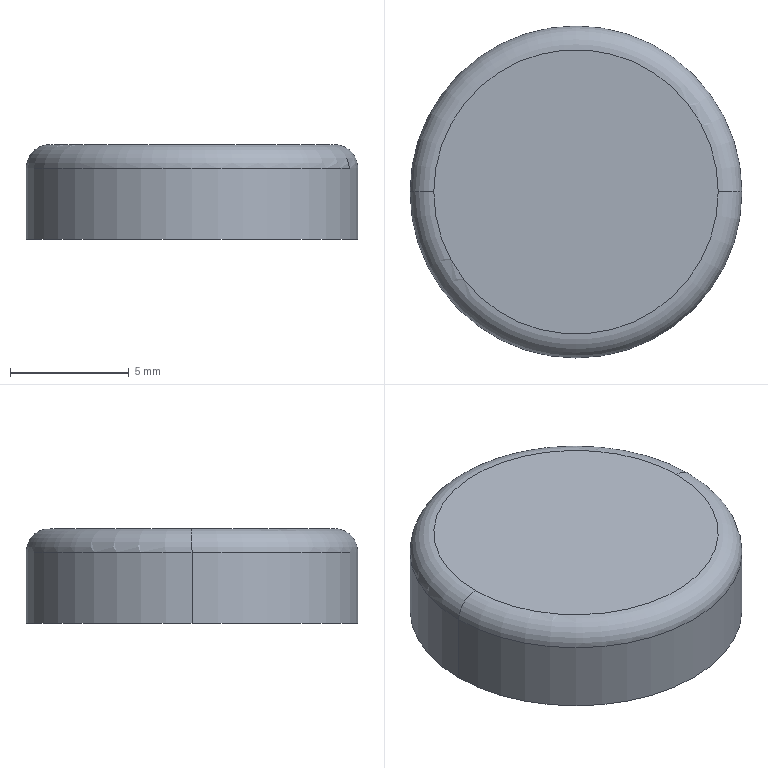Part | STEP file | M8C | 1 solid | 6 faces | box 14 x 14 x 4 mm | volume 606.615 mm3 | torus 2 | cylinder 2 | plane 2 | commonest cylinder face diameters 14 x2
STEP:
#1=CARTESIAN_POINT('',(-7.,0.,3.));
#2=VERTEX_POINT('',#1);
#3=CARTESIAN_POINT('',(7.,0.,3.));
#4=VERTEX_POINT('',#3);
#5=CARTESIAN_POINT('',(0.,0.,3.));
#6=DIRECTION('',(0.,0.,-1.));
#7=DIRECTION('',(1.,0.,0.));
#8=AXIS2_PLACEMENT_3D('',#5,#6,#7);
#9=CIRCLE('',#8,7.);
#10=EDGE_CURVE('',#2,#4,#9,.T.);
#11=ORIENTED_EDGE('',*,*,#10,.F.);
#12=CARTESIAN_POINT('',(-6.,0.,4.));
#13=VERTEX_POINT('',#12);
#14=CARTESIAN_POINT('',(-6.,0.,3.));
#15=DIRECTION('',(0.,1.,0.));
#16=DIRECTION('',(-1.,0.,0.));
#17=AXIS2_PLACEMENT_3D('',#14,#15,#16);
#18=CIRCLE('',#17,1.);
#19=EDGE_CURVE('',#2,#13,#18,.T.);
#20=ORIENTED_EDGE('',*,*,#19,.T.);
#21=CARTESIAN_POINT('',(6.,0.,4.));
#22=VERTEX_POINT('',#21);
#23=CARTESIAN_POINT('',(0.,0.,4.));
#24=DIRECTION('',(0.,0.,1.));
#25=DIRECTION('',(1.,0.,0.));
#26=AXIS2_PLACEMENT_3D('',#23,#24,#25);
#27=CIRCLE('',#26,6.);
#28=EDGE_CURVE('',#22,#13,#27,.T.);
#29=ORIENTED_EDGE('',*,*,#28,.F.);
#30=CARTESIAN_POINT('',(6.,0.,3.));
#31=DIRECTION('',(0.,-1.,0.));
#32=DIRECTION('',(0.,0.,-1.));
#33=AXIS2_PLACEMENT_3D('',#30,#31,#32);
#34=CIRCLE('',#33,1.);
#35=EDGE_CURVE('',#4,#22,#34,.T.);
#36=ORIENTED_EDGE('',*,*,#35,.F.);
#37=EDGE_LOOP('',(#11,#20,#29,#36));
#38=FACE_OUTER_BOUND('',#37,.T.);
#39=CARTESIAN_POINT('',(0.,0.,3.));
#40=DIRECTION('',(0.,0.,1.));
#41=DIRECTION('',(1.,0.,0.));
#42=AXIS2_PLACEMENT_3D('',#39,#40,#41);
#43=TOROIDAL_SURFACE('',#42,6.,1.);
#44=ADVANCED_FACE('',(#38),#43,.T.);
#45=ORIENTED_EDGE('',*,*,#10,.T.);
#46=CARTESIAN_POINT('',(7.,0.,0.));
#47=VERTEX_POINT('',#46);
#48=CARTESIAN_POINT('',(7.,0.,4.));
#49=DIRECTION('',(0.,0.,-1.));
#50=VECTOR('',#49,1000.);
#51=LINE('',#48,#50);
#52=EDGE_CURVE('',#4,#47,#51,.T.);
#53=ORIENTED_EDGE('',*,*,#52,.T.);
#54=CARTESIAN_POINT('',(-7.,0.,0.));
#55=VERTEX_POINT('',#54);
#56=CARTESIAN_POINT('',(0.,0.,0.));
#57=DIRECTION('',(0.,0.,1.));
#58=DIRECTION('',(1.,0.,0.));
#59=AXIS2_PLACEMENT_3D('',#56,#57,#58);
#60=CIRCLE('',#59,7.);
#61=EDGE_CURVE('',#47,#55,#60,.T.);
#62=ORIENTED_EDGE('',*,*,#61,.T.);
#63=CARTESIAN_POINT('',(-7.,0.,4.));
#64=DIRECTION('',(0.,0.,-1.));
#65=VECTOR('',#64,1000.);
#66=LINE('',#63,#65);
#67=EDGE_CURVE('',#2,#55,#66,.T.);
#68=ORIENTED_EDGE('',*,*,#67,.F.);
#69=EDGE_LOOP('',(#45,#53,#62,#68));
#70=FACE_OUTER_BOUND('',#69,.T.);
#71=CARTESIAN_POINT('',(0.,0.,4.));
#72=DIRECTION('',(0.,0.,-1.));
#73=DIRECTION('',(-1.,0.,0.));
#74=AXIS2_PLACEMENT_3D('',#71,#72,#73);
#75=CYLINDRICAL_SURFACE('',#74,7.);
#76=ADVANCED_FACE('',(#70),#75,.T.);
#77=ORIENTED_EDGE('',*,*,#52,.F.);
#78=CARTESIAN_POINT('',(0.,0.,3.));
#79=DIRECTION('',(0.,0.,-1.));
#80=DIRECTION('',(1.,0.,0.));
#81=AXIS2_PLACEMENT_3D('',#78,#79,#80);
#82=CIRCLE('',#81,7.);
#83=EDGE_CURVE('',#4,#2,#82,.T.);
#84=ORIENTED_EDGE('',*,*,#83,.T.);
#85=ORIENTED_EDGE('',*,*,#67,.T.);
#86=CARTESIAN_POINT('',(0.,0.,0.));
#87=DIRECTION('',(0.,0.,1.));
#88=DIRECTION('',(1.,0.,0.));
#89=AXIS2_PLACEMENT_3D('',#86,#87,#88);
#90=CIRCLE('',#89,7.);
#91=EDGE_CURVE('',#55,#47,#90,.T.);
#92=ORIENTED_EDGE('',*,*,#91,.T.);
#93=EDGE_LOOP('',(#77,#84,#85,#92));
#94=FACE_OUTER_BOUND('',#93,.T.);
#95=CARTESIAN_POINT('',(0.,0.,4.));
#96=DIRECTION('',(0.,0.,-1.));
#97=DIRECTION('',(-1.,0.,0.));
#98=AXIS2_PLACEMENT_3D('',#95,#96,#97);
#99=CYLINDRICAL_SURFACE('',#98,7.);
#100=ADVANCED_FACE('',(#94),#99,.T.);
#101=ORIENTED_EDGE('',*,*,#28,.T.);
#102=CARTESIAN_POINT('',(0.,0.,4.));
#103=DIRECTION('',(0.,0.,1.));
#104=DIRECTION('',(1.,0.,0.));
#105=AXIS2_PLACEMENT_3D('',#102,#103,#104);
#106=CIRCLE('',#105,6.);
#107=EDGE_CURVE('',#13,#22,#106,.T.);
#108=ORIENTED_EDGE('',*,*,#107,.T.);
#109=EDGE_LOOP('',(#101,#108));
#110=FACE_OUTER_BOUND('',#109,.T.);
#111=CARTESIAN_POINT('',(0.,0.,4.));
#112=DIRECTION('',(0.,0.,1.));
#113=DIRECTION('',(1.,0.,0.));
#114=AXIS2_PLACEMENT_3D('',#111,#112,#113);
#115=PLANE('',#114);
#116=ADVANCED_FACE('',(#110),#115,.T.);
#117=ORIENTED_EDGE('',*,*,#91,.F.);
#118=ORIENTED_EDGE('',*,*,#61,.F.);
#119=EDGE_LOOP('',(#117,#118));
#120=FACE_OUTER_BOUND('',#119,.T.);
#121=CARTESIAN_POINT('',(0.,0.,0.));
#122=DIRECTION('',(0.,0.,1.));
#123=DIRECTION('',(1.,0.,0.));
#124=AXIS2_PLACEMENT_3D('',#121,#122,#123);
#125=PLANE('',#124);
#126=ADVANCED_FACE('',(#120),#125,.F.);
#127=ORIENTED_EDGE('',*,*,#19,.F.);
#128=ORIENTED_EDGE('',*,*,#83,.F.);
#129=ORIENTED_EDGE('',*,*,#35,.T.);
#130=ORIENTED_EDGE('',*,*,#107,.F.);
#131=EDGE_LOOP('',(#127,#128,#129,#130));
#132=FACE_OUTER_BOUND('',#131,.T.);
#133=CARTESIAN_POINT('',(0.,0.,3.));
#134=DIRECTION('',(0.,0.,1.));
#135=DIRECTION('',(1.,0.,0.));
#136=AXIS2_PLACEMENT_3D('',#133,#134,#135);
#137=TOROIDAL_SURFACE('',#136,6.,1.);
#138=ADVANCED_FACE('',(#132),#137,.T.);
#139=CLOSED_SHELL('',(#44,#76,#100,#116,#126,#138));
#140=MANIFOLD_SOLID_BREP('',#139);
#141=CARTESIAN_POINT('',(0.,0.,0.));
#142=DIRECTION('',(0.,0.,1.));
#143=DIRECTION('',(1.,0.,0.));
#144=AXIS2_PLACEMENT_3D('',#141,#142,#143);
#145=(LENGTH_UNIT()NAMED_UNIT(*)SI_UNIT(.MILLI.,.METRE.));
#146=UNCERTAINTY_MEASURE_WITH_UNIT(LENGTH_MEASURE(0.00001),#145,'','');
#147=(NAMED_UNIT(*)PLANE_ANGLE_UNIT()SI_UNIT($,.RADIAN.));
#148=(NAMED_UNIT(*)SI_UNIT($,.STERADIAN.)SOLID_ANGLE_UNIT());
#149=(GEOMETRIC_REPRESENTATION_CONTEXT(3)GLOBAL_UNCERTAINTY_ASSIGNED_CONTEXT((#146))GLOBAL_UNIT_ASSIGNED_CONTEXT((#145,#147,#148))REPRESENTATION_CONTEXT('',''));
#150=ADVANCED_BREP_SHAPE_REPRESENTATION('',(#140,#144),#149);